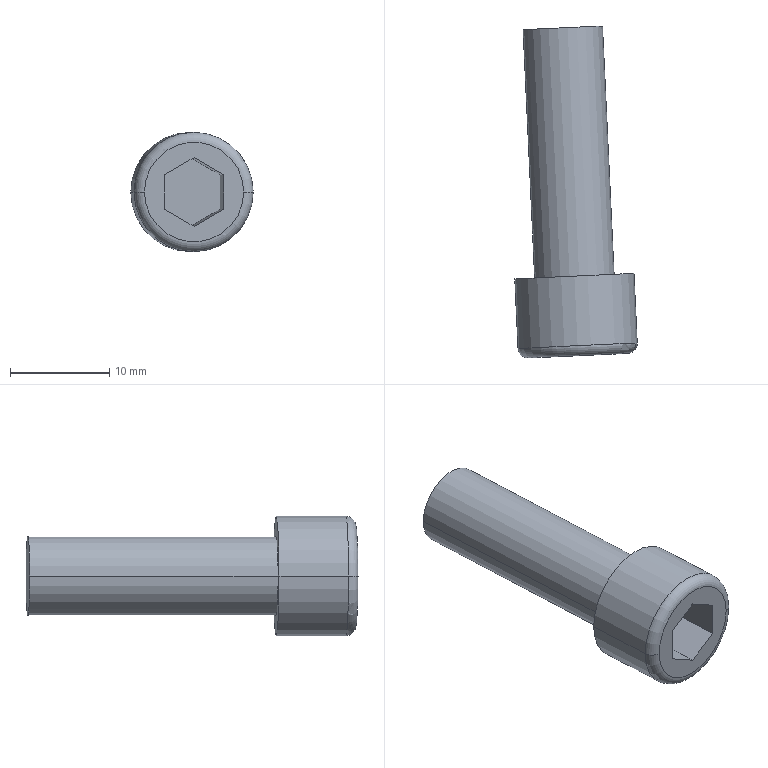Part | SolidWorks | features BaseBody 1 | 1 solid | 16 faces | box 12.314 x 33.385 x 12 mm | volume 1904 mm3 | plane 10 | cylinder 4 | torus 2 | commonest cylinder face diameters 8 x2 12 x2
STEP:
#1=CARTESIAN_POINT('',(98.765,977.523,327.607));
#2=VERTEX_POINT('',#1);
#3=CARTESIAN_POINT('',(97.719,978.476,327.607));
#4=VERTEX_POINT('',#3);
#5=CARTESIAN_POINT('',(98.718,978.522,327.607));
#6=DIRECTION('',(0.,0.,-1.));
#7=DIRECTION('',(-0.9989,-0.04661,0.));
#8=AXIS2_PLACEMENT_3D('',#5,#6,#7);
#9=CIRCLE('',#8,1.);
#10=EDGE_CURVE('',#2,#4,#9,.T.);
#11=ORIENTED_EDGE('',*,*,#10,.F.);
#12=CARTESIAN_POINT('',(108.754,977.99,327.607));
#13=VERTEX_POINT('',#12);
#14=CARTESIAN_POINT('',(103.759,977.757,327.607));
#15=DIRECTION('',(0.04661,-0.9989,0.));
#16=DIRECTION('',(0.9989,0.04661,0.));
#17=AXIS2_PLACEMENT_3D('',#14,#15,#16);
#18=CIRCLE('',#17,5.);
#19=EDGE_CURVE('',#13,#2,#18,.T.);
#20=ORIENTED_EDGE('',*,*,#19,.F.);
#21=CARTESIAN_POINT('',(109.706,979.035,327.607));
#22=VERTEX_POINT('',#21);
#23=CARTESIAN_POINT('',(108.707,978.988,327.607));
#24=DIRECTION('',(0.,0.,1.));
#25=DIRECTION('',(0.04661,-0.9989,0.));
#26=AXIS2_PLACEMENT_3D('',#23,#24,#25);
#27=CIRCLE('',#26,1.);
#28=EDGE_CURVE('',#13,#22,#27,.T.);
#29=ORIENTED_EDGE('',*,*,#28,.T.);
#30=CARTESIAN_POINT('',(103.713,978.755,327.607));
#31=DIRECTION('',(-0.04661,0.9989,0.));
#32=DIRECTION('',(0.9989,0.04661,0.));
#33=AXIS2_PLACEMENT_3D('',#30,#31,#32);
#34=CIRCLE('',#33,6.);
#35=EDGE_CURVE('',#4,#22,#34,.T.);
#36=ORIENTED_EDGE('',*,*,#35,.F.);
#37=EDGE_LOOP('',(#11,#20,#29,#36));
#38=FACE_OUTER_BOUND('',#37,.T.);
#39=CARTESIAN_POINT('',(103.713,978.755,327.607));
#40=DIRECTION('',(-0.04661,0.9989,0.));
#41=DIRECTION('',(-0.9989,-0.04661,0.));
#42=AXIS2_PLACEMENT_3D('',#39,#40,#41);
#43=TOROIDAL_SURFACE('',#42,5.,1.);
#44=ADVANCED_FACE('',(#38),#43,.T.);
#45=CARTESIAN_POINT('',(106.383,985.888,325.875));
#46=VERTEX_POINT('',#45);
#47=CARTESIAN_POINT('',(103.386,985.748,324.143));
#48=VERTEX_POINT('',#47);
#49=CARTESIAN_POINT('',(110.655,986.087,328.344));
#50=DIRECTION('',(-0.8651,-0.04037,-0.5));
#51=VECTOR('',#50,1000.);
#52=LINE('',#49,#51);
#53=EDGE_CURVE('',#46,#48,#52,.T.);
#54=ORIENTED_EDGE('',*,*,#53,.F.);
#55=CARTESIAN_POINT('',(106.383,985.888,329.339));
#56=VERTEX_POINT('',#55);
#57=CARTESIAN_POINT('',(106.383,985.888,340.948));
#58=DIRECTION('',(0.,0.,-1.));
#59=VECTOR('',#58,1000.);
#60=LINE('',#57,#59);
#61=EDGE_CURVE('',#56,#46,#60,.T.);
#62=ORIENTED_EDGE('',*,*,#61,.F.);
#63=CARTESIAN_POINT('',(103.386,985.748,331.071));
#64=VERTEX_POINT('',#63);
#65=CARTESIAN_POINT('',(99.114,985.548,333.54));
#66=DIRECTION('',(0.8651,0.04037,-0.5));
#67=VECTOR('',#66,1000.);
#68=LINE('',#65,#67);
#69=EDGE_CURVE('',#64,#56,#68,.T.);
#70=ORIENTED_EDGE('',*,*,#69,.F.);
#71=CARTESIAN_POINT('',(100.39,985.608,329.339));
#72=VERTEX_POINT('',#71);
#73=CARTESIAN_POINT('',(107.659,985.947,333.54));
#74=DIRECTION('',(0.8651,0.04037,0.5));
#75=VECTOR('',#74,1000.);
#76=LINE('',#73,#75);
#77=EDGE_CURVE('',#72,#64,#76,.T.);
#78=ORIENTED_EDGE('',*,*,#77,.F.);
#79=CARTESIAN_POINT('',(100.39,985.608,325.875));
#80=VERTEX_POINT('',#79);
#81=CARTESIAN_POINT('',(100.39,985.608,340.948));
#82=DIRECTION('',(0.,0.,1.));
#83=VECTOR('',#82,1000.);
#84=LINE('',#81,#83);
#85=EDGE_CURVE('',#80,#72,#84,.T.);
#86=ORIENTED_EDGE('',*,*,#85,.F.);
#87=CARTESIAN_POINT('',(96.117,985.409,328.344));
#88=DIRECTION('',(-0.8651,-0.04037,0.5));
#89=VECTOR('',#88,1000.);
#90=LINE('',#87,#89);
#91=EDGE_CURVE('',#48,#80,#90,.T.);
#92=ORIENTED_EDGE('',*,*,#91,.F.);
#93=EDGE_LOOP('',(#54,#62,#70,#78,#86,#92));
#94=FACE_OUTER_BOUND('',#93,.T.);
#95=CARTESIAN_POINT('',(103.386,985.748,340.948));
#96=DIRECTION('',(-0.04661,0.9989,0.));
#97=DIRECTION('',(0.,0.,1.));
#98=AXIS2_PLACEMENT_3D('',#95,#96,#97);
#99=PLANE('',#98);
#100=ADVANCED_FACE('',(#94),#99,.F.);
#101=CARTESIAN_POINT('',(103.759,977.757,331.071));
#102=VERTEX_POINT('',#101);
#103=CARTESIAN_POINT('',(106.756,977.896,329.339));
#104=VERTEX_POINT('',#103);
#105=CARTESIAN_POINT('',(99.487,977.557,333.54));
#106=DIRECTION('',(0.8651,0.04037,-0.5));
#107=VECTOR('',#106,1000.);
#108=LINE('',#105,#107);
#109=EDGE_CURVE('',#102,#104,#108,.T.);
#110=ORIENTED_EDGE('',*,*,#109,.T.);
#111=CARTESIAN_POINT('',(106.756,977.896,325.875));
#112=VERTEX_POINT('',#111);
#113=CARTESIAN_POINT('',(106.756,977.896,340.948));
#114=DIRECTION('',(0.,0.,-1.));
#115=VECTOR('',#114,1000.);
#116=LINE('',#113,#115);
#117=EDGE_CURVE('',#104,#112,#116,.T.);
#118=ORIENTED_EDGE('',*,*,#117,.T.);
#119=CARTESIAN_POINT('',(103.759,977.757,324.143));
#120=VERTEX_POINT('',#119);
#121=CARTESIAN_POINT('',(111.028,978.096,328.344));
#122=DIRECTION('',(-0.8651,-0.04037,-0.5));
#123=VECTOR('',#122,1000.);
#124=LINE('',#121,#123);
#125=EDGE_CURVE('',#112,#120,#124,.T.);
#126=ORIENTED_EDGE('',*,*,#125,.T.);
#127=CARTESIAN_POINT('',(100.763,977.617,325.875));
#128=VERTEX_POINT('',#127);
#129=CARTESIAN_POINT('',(96.49,977.417,328.344));
#130=DIRECTION('',(-0.8651,-0.04037,0.5));
#131=VECTOR('',#130,1000.);
#132=LINE('',#129,#131);
#133=EDGE_CURVE('',#120,#128,#132,.T.);
#134=ORIENTED_EDGE('',*,*,#133,.T.);
#135=CARTESIAN_POINT('',(100.763,977.617,329.339));
#136=VERTEX_POINT('',#135);
#137=CARTESIAN_POINT('',(100.763,977.617,340.948));
#138=DIRECTION('',(0.,0.,1.));
#139=VECTOR('',#138,1000.);
#140=LINE('',#137,#139);
#141=EDGE_CURVE('',#128,#136,#140,.T.);
#142=ORIENTED_EDGE('',*,*,#141,.T.);
#143=CARTESIAN_POINT('',(108.032,977.956,333.54));
#144=DIRECTION('',(0.8651,0.04037,0.5));
#145=VECTOR('',#144,1000.);
#146=LINE('',#143,#145);
#147=EDGE_CURVE('',#136,#102,#146,.T.);
#148=ORIENTED_EDGE('',*,*,#147,.T.);
#149=EDGE_LOOP('',(#110,#118,#126,#134,#142,#148));
#150=FACE_BOUND('',#149,.T.);
#151=ORIENTED_EDGE('',*,*,#19,.T.);
#152=CARTESIAN_POINT('',(103.759,977.757,327.607));
#153=DIRECTION('',(0.04661,-0.9989,0.));
#154=DIRECTION('',(0.9989,0.04661,0.));
#155=AXIS2_PLACEMENT_3D('',#152,#153,#154);
#156=CIRCLE('',#155,5.);
#157=EDGE_CURVE('',#2,#13,#156,.T.);
#158=ORIENTED_EDGE('',*,*,#157,.T.);
#159=EDGE_LOOP('',(#151,#158));
#160=FACE_OUTER_BOUND('',#159,.T.);
#161=CARTESIAN_POINT('',(103.759,977.757,340.948));
#162=DIRECTION('',(-0.04661,0.9989,0.));
#163=DIRECTION('',(0.,0.,1.));
#164=AXIS2_PLACEMENT_3D('',#161,#162,#163);
#165=PLANE('',#164);
#166=ADVANCED_FACE('',(#150,#160),#165,.F.);
#167=CARTESIAN_POINT('',(97.393,985.468,327.607));
#168=VERTEX_POINT('',#167);
#169=CARTESIAN_POINT('',(97.766,977.477,327.607));
#170=DIRECTION('',(-0.04661,0.9989,0.));
#171=VECTOR('',#170,1000.);
#172=LINE('',#169,#171);
#173=EDGE_CURVE('',#4,#168,#172,.T.);
#174=ORIENTED_EDGE('',*,*,#173,.F.);
#175=ORIENTED_EDGE('',*,*,#35,.T.);
#176=CARTESIAN_POINT('',(109.38,986.027,327.607));
#177=VERTEX_POINT('',#176);
#178=CARTESIAN_POINT('',(109.753,978.036,327.607));
#179=DIRECTION('',(-0.04661,0.9989,0.));
#180=VECTOR('',#179,1000.);
#181=LINE('',#178,#180);
#182=EDGE_CURVE('',#22,#177,#181,.T.);
#183=ORIENTED_EDGE('',*,*,#182,.T.);
#184=CARTESIAN_POINT('',(103.386,985.748,327.607));
#185=DIRECTION('',(-0.04661,0.9989,0.));
#186=DIRECTION('',(0.9989,0.04661,0.));
#187=AXIS2_PLACEMENT_3D('',#184,#185,#186);
#188=CIRCLE('',#187,6.);
#189=EDGE_CURVE('',#168,#177,#188,.T.);
#190=ORIENTED_EDGE('',*,*,#189,.F.);
#191=EDGE_LOOP('',(#174,#175,#183,#190));
#192=FACE_OUTER_BOUND('',#191,.T.);
#193=CARTESIAN_POINT('',(103.759,977.757,327.607));
#194=DIRECTION('',(-0.04661,0.9989,0.));
#195=DIRECTION('',(-0.9989,-0.04661,0.));
#196=AXIS2_PLACEMENT_3D('',#193,#194,#195);
#197=CYLINDRICAL_SURFACE('',#196,6.);
#198=ADVANCED_FACE('',(#192),#197,.T.);
#199=ORIENTED_EDGE('',*,*,#53,.T.);
#200=CARTESIAN_POINT('',(103.759,977.757,324.143));
#201=DIRECTION('',(-0.04661,0.9989,0.));
#202=VECTOR('',#201,1000.);
#203=LINE('',#200,#202);
#204=EDGE_CURVE('',#120,#48,#203,.T.);
#205=ORIENTED_EDGE('',*,*,#204,.F.);
#206=ORIENTED_EDGE('',*,*,#125,.F.);
#207=CARTESIAN_POINT('',(106.756,977.896,325.875));
#208=DIRECTION('',(-0.04661,0.9989,0.));
#209=VECTOR('',#208,1000.);
#210=LINE('',#207,#209);
#211=EDGE_CURVE('',#112,#46,#210,.T.);
#212=ORIENTED_EDGE('',*,*,#211,.T.);
#213=EDGE_LOOP('',(#199,#205,#206,#212));
#214=FACE_OUTER_BOUND('',#213,.T.);
#215=CARTESIAN_POINT('',(111.028,978.096,328.344));
#216=DIRECTION('',(0.4995,0.02331,-0.866));
#217=DIRECTION('',(0.,-0.9996,-0.0269));
#218=AXIS2_PLACEMENT_3D('',#215,#216,#217);
#219=PLANE('',#218);
#220=ADVANCED_FACE('',(#214),#219,.F.);
#221=ORIENTED_EDGE('',*,*,#91,.T.);
#222=CARTESIAN_POINT('',(100.763,977.617,325.875));
#223=DIRECTION('',(-0.04661,0.9989,0.));
#224=VECTOR('',#223,1000.);
#225=LINE('',#222,#224);
#226=EDGE_CURVE('',#128,#80,#225,.T.);
#227=ORIENTED_EDGE('',*,*,#226,.F.);
#228=ORIENTED_EDGE('',*,*,#133,.F.);
#229=ORIENTED_EDGE('',*,*,#204,.T.);
#230=EDGE_LOOP('',(#221,#227,#228,#229));
#231=FACE_OUTER_BOUND('',#230,.T.);
#232=CARTESIAN_POINT('',(96.49,977.417,328.344));
#233=DIRECTION('',(-0.4995,-0.02331,-0.866));
#234=DIRECTION('',(-0.8663,0.,0.4996));
#235=AXIS2_PLACEMENT_3D('',#232,#233,#234);
#236=PLANE('',#235);
#237=ADVANCED_FACE('',(#231),#236,.F.);
#238=ORIENTED_EDGE('',*,*,#85,.T.);
#239=CARTESIAN_POINT('',(100.763,977.617,329.339));
#240=DIRECTION('',(-0.04661,0.9989,0.));
#241=VECTOR('',#240,1000.);
#242=LINE('',#239,#241);
#243=EDGE_CURVE('',#136,#72,#242,.T.);
#244=ORIENTED_EDGE('',*,*,#243,.F.);
#245=ORIENTED_EDGE('',*,*,#141,.F.);
#246=ORIENTED_EDGE('',*,*,#226,.T.);
#247=EDGE_LOOP('',(#238,#244,#245,#246));
#248=FACE_OUTER_BOUND('',#247,.T.);
#249=CARTESIAN_POINT('',(100.763,977.617,340.948));
#250=DIRECTION('',(-0.9989,-0.04661,0.));
#251=DIRECTION('',(-0.04661,0.9989,0.));
#252=AXIS2_PLACEMENT_3D('',#249,#250,#251);
#253=PLANE('',#252);
#254=ADVANCED_FACE('',(#248),#253,.F.);
#255=ORIENTED_EDGE('',*,*,#77,.T.);
#256=CARTESIAN_POINT('',(103.759,977.757,331.071));
#257=DIRECTION('',(-0.04661,0.9989,0.));
#258=VECTOR('',#257,1000.);
#259=LINE('',#256,#258);
#260=EDGE_CURVE('',#102,#64,#259,.T.);
#261=ORIENTED_EDGE('',*,*,#260,.F.);
#262=ORIENTED_EDGE('',*,*,#147,.F.);
#263=ORIENTED_EDGE('',*,*,#243,.T.);
#264=EDGE_LOOP('',(#255,#261,#262,#263));
#265=FACE_OUTER_BOUND('',#264,.T.);
#266=CARTESIAN_POINT('',(108.032,977.956,333.54));
#267=DIRECTION('',(-0.4995,-0.02331,0.866));
#268=DIRECTION('',(-0.04661,0.9989,0.));
#269=AXIS2_PLACEMENT_3D('',#266,#267,#268);
#270=PLANE('',#269);
#271=ADVANCED_FACE('',(#265),#270,.F.);
#272=ORIENTED_EDGE('',*,*,#69,.T.);
#273=CARTESIAN_POINT('',(106.756,977.896,329.339));
#274=DIRECTION('',(-0.04661,0.9989,0.));
#275=VECTOR('',#274,1000.);
#276=LINE('',#273,#275);
#277=EDGE_CURVE('',#104,#56,#276,.T.);
#278=ORIENTED_EDGE('',*,*,#277,.F.);
#279=ORIENTED_EDGE('',*,*,#109,.F.);
#280=ORIENTED_EDGE('',*,*,#260,.T.);
#281=EDGE_LOOP('',(#272,#278,#279,#280));
#282=FACE_OUTER_BOUND('',#281,.T.);
#283=CARTESIAN_POINT('',(99.487,977.557,333.54));
#284=DIRECTION('',(0.4995,0.02331,0.866));
#285=DIRECTION('',(0.04661,-0.9989,0.));
#286=AXIS2_PLACEMENT_3D('',#283,#284,#285);
#287=PLANE('',#286);
#288=ADVANCED_FACE('',(#282),#287,.F.);
#289=ORIENTED_EDGE('',*,*,#61,.T.);
#290=ORIENTED_EDGE('',*,*,#211,.F.);
#291=ORIENTED_EDGE('',*,*,#117,.F.);
#292=ORIENTED_EDGE('',*,*,#277,.T.);
#293=EDGE_LOOP('',(#289,#290,#291,#292));
#294=FACE_OUTER_BOUND('',#293,.T.);
#295=CARTESIAN_POINT('',(106.756,977.896,340.948));
#296=DIRECTION('',(0.9989,0.04661,0.));
#297=DIRECTION('',(0.,0.,-1.));
#298=AXIS2_PLACEMENT_3D('',#295,#296,#297);
#299=PLANE('',#298);
#300=ADVANCED_FACE('',(#294),#299,.F.);
#301=CARTESIAN_POINT('',(99.391,985.561,327.607));
#302=VERTEX_POINT('',#301);
#303=CARTESIAN_POINT('',(107.382,985.934,327.607));
#304=VERTEX_POINT('',#303);
#305=CARTESIAN_POINT('',(103.386,985.748,327.607));
#306=DIRECTION('',(-0.04661,0.9989,0.));
#307=DIRECTION('',(0.9989,0.04661,0.));
#308=AXIS2_PLACEMENT_3D('',#305,#306,#307);
#309=CIRCLE('',#308,4.);
#310=EDGE_CURVE('',#302,#304,#309,.T.);
#311=ORIENTED_EDGE('',*,*,#310,.F.);
#312=CARTESIAN_POINT('',(103.386,985.748,327.607));
#313=DIRECTION('',(-0.04661,0.9989,0.));
#314=DIRECTION('',(0.9989,0.04661,0.));
#315=AXIS2_PLACEMENT_3D('',#312,#313,#314);
#316=CIRCLE('',#315,4.);
#317=EDGE_CURVE('',#304,#302,#316,.T.);
#318=ORIENTED_EDGE('',*,*,#317,.F.);
#319=EDGE_LOOP('',(#311,#318));
#320=FACE_BOUND('',#319,.T.);
#321=CARTESIAN_POINT('',(103.386,985.748,327.607));
#322=DIRECTION('',(-0.04661,0.9989,0.));
#323=DIRECTION('',(0.9989,0.04661,0.));
#324=AXIS2_PLACEMENT_3D('',#321,#322,#323);
#325=CIRCLE('',#324,6.);
#326=EDGE_CURVE('',#177,#168,#325,.T.);
#327=ORIENTED_EDGE('',*,*,#326,.T.);
#328=ORIENTED_EDGE('',*,*,#189,.T.);
#329=EDGE_LOOP('',(#327,#328));
#330=FACE_OUTER_BOUND('',#329,.T.);
#331=CARTESIAN_POINT('',(103.386,985.748,340.948));
#332=DIRECTION('',(-0.04661,0.9989,0.));
#333=DIRECTION('',(0.,0.,1.));
#334=AXIS2_PLACEMENT_3D('',#331,#332,#333);
#335=PLANE('',#334);
#336=ADVANCED_FACE('',(#320,#330),#335,.T.);
#337=CARTESIAN_POINT('',(98.225,1010.534,327.607));
#338=VERTEX_POINT('',#337);
#339=CARTESIAN_POINT('',(106.217,1010.907,327.607));
#340=VERTEX_POINT('',#339);
#341=CARTESIAN_POINT('',(102.221,1010.721,327.607));
#342=DIRECTION('',(-0.04661,0.9989,0.));
#343=DIRECTION('',(0.9989,0.04661,0.));
#344=AXIS2_PLACEMENT_3D('',#341,#342,#343);
#345=CIRCLE('',#344,4.);
#346=EDGE_CURVE('',#338,#340,#345,.T.);
#347=ORIENTED_EDGE('',*,*,#346,.T.);
#348=CARTESIAN_POINT('',(102.221,1010.721,327.607));
#349=DIRECTION('',(-0.04661,0.9989,0.));
#350=DIRECTION('',(0.9989,0.04661,0.));
#351=AXIS2_PLACEMENT_3D('',#348,#349,#350);
#352=CIRCLE('',#351,4.);
#353=EDGE_CURVE('',#340,#338,#352,.T.);
#354=ORIENTED_EDGE('',*,*,#353,.T.);
#355=EDGE_LOOP('',(#347,#354));
#356=FACE_OUTER_BOUND('',#355,.T.);
#357=CARTESIAN_POINT('',(102.221,1010.721,340.948));
#358=DIRECTION('',(-0.04661,0.9989,0.));
#359=DIRECTION('',(0.,0.,1.));
#360=AXIS2_PLACEMENT_3D('',#357,#358,#359);
#361=PLANE('',#360);
#362=ADVANCED_FACE('',(#356),#361,.T.);
#363=CARTESIAN_POINT('',(106.217,1010.907,327.607));
#364=DIRECTION('',(0.04661,-0.9989,0.));
#365=VECTOR('',#364,1000.);
#366=LINE('',#363,#365);
#367=EDGE_CURVE('',#340,#304,#366,.T.);
#368=ORIENTED_EDGE('',*,*,#367,.F.);
#369=ORIENTED_EDGE('',*,*,#346,.F.);
#370=CARTESIAN_POINT('',(98.225,1010.534,327.607));
#371=DIRECTION('',(0.04661,-0.9989,0.));
#372=VECTOR('',#371,1000.);
#373=LINE('',#370,#372);
#374=EDGE_CURVE('',#338,#302,#373,.T.);
#375=ORIENTED_EDGE('',*,*,#374,.T.);
#376=ORIENTED_EDGE('',*,*,#310,.T.);
#377=EDGE_LOOP('',(#368,#369,#375,#376));
#378=FACE_OUTER_BOUND('',#377,.T.);
#379=CARTESIAN_POINT('',(102.221,1010.721,327.607));
#380=DIRECTION('',(0.04661,-0.9989,0.));
#381=DIRECTION('',(0.9989,0.04661,0.));
#382=AXIS2_PLACEMENT_3D('',#379,#380,#381);
#383=CYLINDRICAL_SURFACE('',#382,4.);
#384=ADVANCED_FACE('',(#378),#383,.T.);
#385=ORIENTED_EDGE('',*,*,#353,.F.);
#386=ORIENTED_EDGE('',*,*,#367,.T.);
#387=ORIENTED_EDGE('',*,*,#317,.T.);
#388=ORIENTED_EDGE('',*,*,#374,.F.);
#389=EDGE_LOOP('',(#385,#386,#387,#388));
#390=FACE_OUTER_BOUND('',#389,.T.);
#391=CARTESIAN_POINT('',(102.221,1010.721,327.607));
#392=DIRECTION('',(0.04661,-0.9989,0.));
#393=DIRECTION('',(0.9989,0.04661,0.));
#394=AXIS2_PLACEMENT_3D('',#391,#392,#393);
#395=CYLINDRICAL_SURFACE('',#394,4.);
#396=ADVANCED_FACE('',(#390),#395,.T.);
#397=CARTESIAN_POINT('',(103.713,978.755,327.607));
#398=DIRECTION('',(-0.04661,0.9989,0.));
#399=DIRECTION('',(0.9989,0.04661,0.));
#400=AXIS2_PLACEMENT_3D('',#397,#398,#399);
#401=CIRCLE('',#400,6.);
#402=EDGE_CURVE('',#22,#4,#401,.T.);
#403=ORIENTED_EDGE('',*,*,#402,.T.);
#404=ORIENTED_EDGE('',*,*,#173,.T.);
#405=ORIENTED_EDGE('',*,*,#326,.F.);
#406=ORIENTED_EDGE('',*,*,#182,.F.);
#407=EDGE_LOOP('',(#403,#404,#405,#406));
#408=FACE_OUTER_BOUND('',#407,.T.);
#409=CARTESIAN_POINT('',(103.759,977.757,327.607));
#410=DIRECTION('',(-0.04661,0.9989,0.));
#411=DIRECTION('',(-0.9989,-0.04661,0.));
#412=AXIS2_PLACEMENT_3D('',#409,#410,#411);
#413=CYLINDRICAL_SURFACE('',#412,6.);
#414=ADVANCED_FACE('',(#408),#413,.T.);
#415=ORIENTED_EDGE('',*,*,#157,.F.);
#416=ORIENTED_EDGE('',*,*,#10,.T.);
#417=ORIENTED_EDGE('',*,*,#402,.F.);
#418=ORIENTED_EDGE('',*,*,#28,.F.);
#419=EDGE_LOOP('',(#415,#416,#417,#418));
#420=FACE_OUTER_BOUND('',#419,.T.);
#421=CARTESIAN_POINT('',(103.713,978.755,327.607));
#422=DIRECTION('',(-0.04661,0.9989,0.));
#423=DIRECTION('',(-0.9989,-0.04661,0.));
#424=AXIS2_PLACEMENT_3D('',#421,#422,#423);
#425=TOROIDAL_SURFACE('',#424,5.,1.);
#426=ADVANCED_FACE('',(#420),#425,.T.);
#427=CLOSED_SHELL('',(#44,#100,#166,#198,#220,#237,#254,#271,#288,#300,#336,#362,#384,#396,#414,#426));
#428=MANIFOLD_SOLID_BREP('',#427);
#429=CARTESIAN_POINT('',(0.,0.,0.));
#430=DIRECTION('',(0.,0.,1.));
#431=DIRECTION('',(1.,0.,0.));
#432=AXIS2_PLACEMENT_3D('',#429,#430,#431);
#433=(LENGTH_UNIT()NAMED_UNIT(*)SI_UNIT(.MILLI.,.METRE.));
#434=UNCERTAINTY_MEASURE_WITH_UNIT(LENGTH_MEASURE(0.00001),#433,'','');
#435=(NAMED_UNIT(*)PLANE_ANGLE_UNIT()SI_UNIT($,.RADIAN.));
#436=(NAMED_UNIT(*)SI_UNIT($,.STERADIAN.)SOLID_ANGLE_UNIT());
#437=(GEOMETRIC_REPRESENTATION_CONTEXT(3)GLOBAL_UNCERTAINTY_ASSIGNED_CONTEXT((#434))GLOBAL_UNIT_ASSIGNED_CONTEXT((#433,#435,#436))REPRESENTATION_CONTEXT('',''));
#438=ADVANCED_BREP_SHAPE_REPRESENTATION('',(#428,#432),#437);